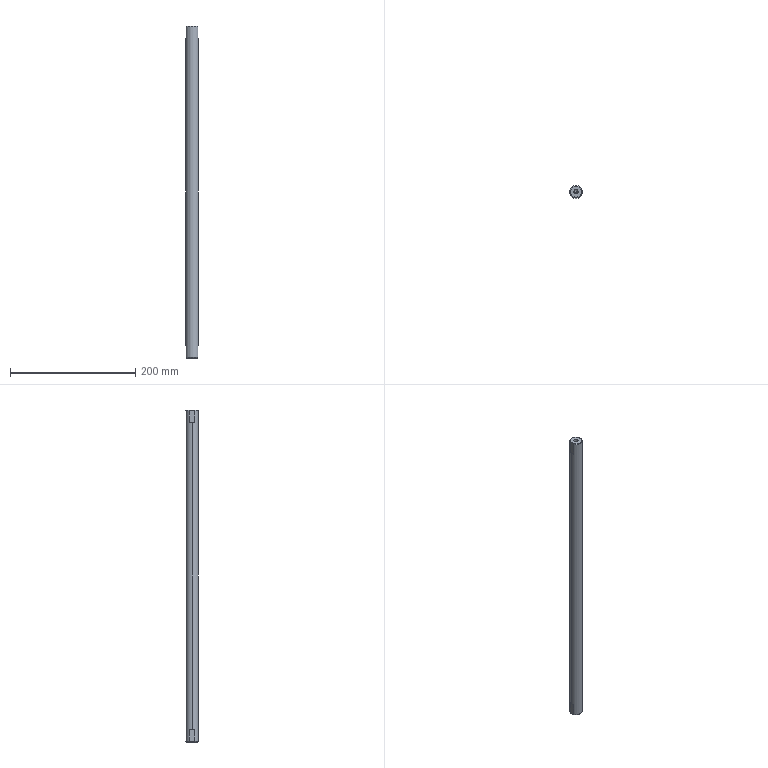Part | STEP file | 1 solid | 24 faces | box 20 x 20 x 530 mm | volume 164323 mm3 | plane 10 | cone 8 | cylinder 6 | commonest cylinder face diameters 6.8 x4 20 x2